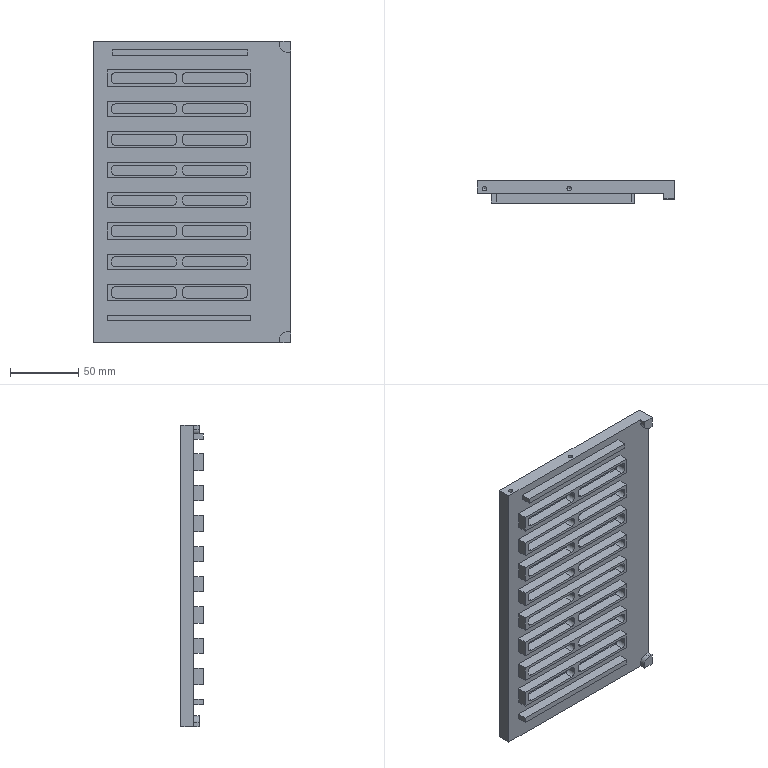NC program | NX | posted with a generic post | part box 144.5 x 16.5 x 221 mm
Lines 1 to 113 of 11164:
N10 G17 G21 G94 G90
(FLOOR_WALL_2 , TOOL : D63面刀)
N12 T01 M6
N14 G54
N16 G17 G0 G90 X-147. Y56.5 B0. C0. S3500 M3
N18 G43 Z20. H1
N20 Z4.517 B-180. C-180.
N22 G94 G1 Z2.517 F1000.
N24 X-142.
N26 X142.
N28 Y21.983
N30 X-142.
N32 Y-12.533
N34 X142.
N36 Y-47.05
N38 X-142.
N40 X-147.
N42 Z4.517
N44 G0 Z20.
N46 Y56.5
N48 Z4.033
N50 G1 Z2.033
N52 X-142.
N54 X142.
N56 Y21.983
N58 X-142.
N60 Y-12.533
N62 X142.
N64 Y-47.05
N66 X-142.
N68 X-147.
N70 Z4.033
N72 G0 Z20.
N74 Y56.5
N76 Z3.55
N78 G1 Z1.55
N80 X-142.
N82 X142.
N84 Y21.983
N86 X-142.
N88 Y-12.533
N90 X142.
N92 Y-47.05
N94 X-142.
N96 X-147.
N98 Z3.55
N100 G0 Z20.
N102 Y56.5
N104 Z3.067
N106 G1 Z1.067
N108 X-142.
N110 X142.
N112 Y21.983
N114 X-142.
N116 Y-12.533
N118 X142.
N120 Y-47.05
N122 X-142.
N124 X-147.
N126 Z3.067
N128 G0 Z20.
N130 Y56.5
N132 Z2.583
N134 G1 Z0.583
N136 X-142.
N138 X142.
N140 Y21.983
N142 X-142.
N144 Y-12.533
N146 X142.
N148 Y-47.05
N150 X-142.
N152 X-147.
N154 Z2.583
N156 G0 Z20.
N158 Y56.5
N160 Z2.1
N162 G1 Z0.1
N164 X-142.
N166 X142.
N168 Y21.983
N170 X-142.
N172 Y-12.533
N174 X142.
N176 Y-47.05
N178 X-142.
N180 X-147.
N182 Z2.1
N184 G0 Z20.
(FLOOR_WALL_2_COPY , TOOL : D63面刀)
N186 X94.75 Y108.75
N188 Z2.
N190 G1 Z0. F800.
N192 Y103.75
N194 Y-103.75
N196 X49.737
N198 Y103.75
N200 X4.725
N202 Y-103.75
N204 X-40.287
N206 Y103.75
N208 X-85.3
N210 Y-103.75
N212 Y-108.75
N214 Z2.
N216 G0 Z20.
N218 M5